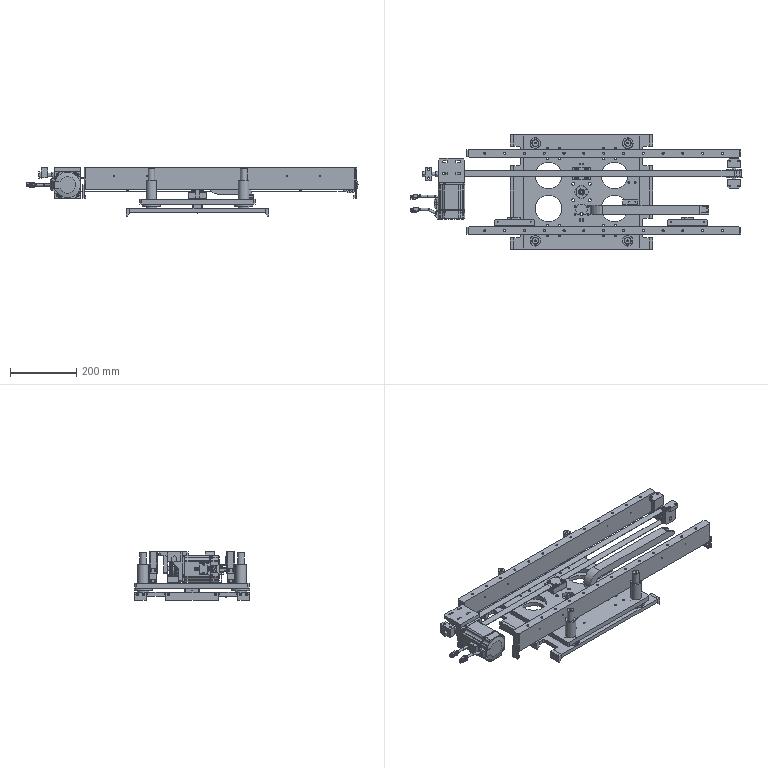Part | NX | 68 solids | 2883 faces | box 1006 x 350 x 147 mm | volume 7052344 mm3 | plane 1532 | cylinder 1098 | cone 143 | spline 110 | commonest cylinder face diameters 0.8 x109 1.2 x108 4.2 x62 8 x60 10 x60 40.6 x57